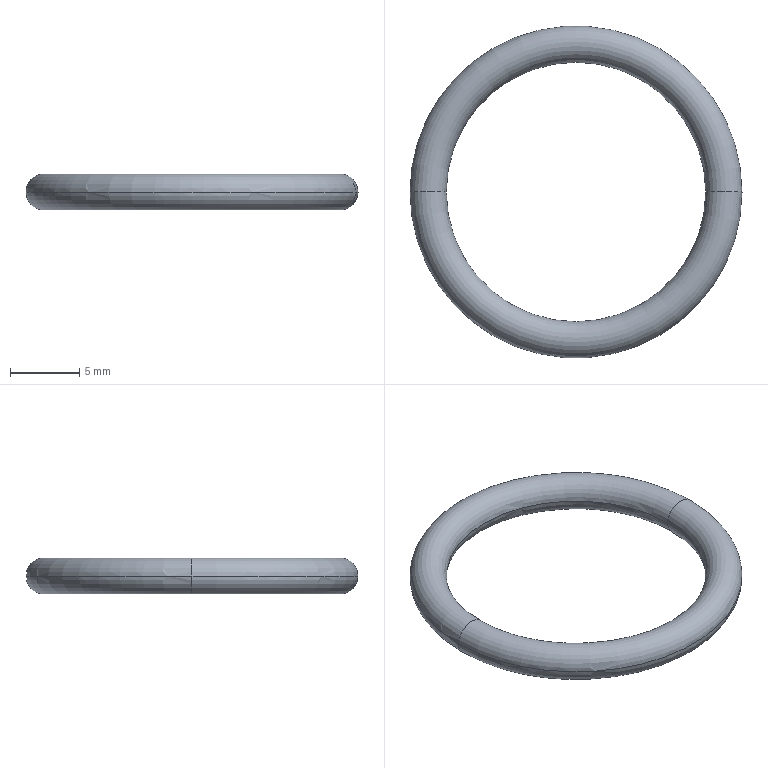Part | NX | features REVOLVE1 2 | 1 solid | 4 faces | box 23.952 x 23.952 x 2.616 mm | volume 360.325 mm3 | torus 4
STEP:
#1=CARTESIAN_POINT('',(-11.976,0.,0.));
#2=VERTEX_POINT('',#1);
#3=CARTESIAN_POINT('',(-9.36,0.,0.));
#4=VERTEX_POINT('',#3);
#5=CARTESIAN_POINT('',(-10.668,0.,0.));
#6=DIRECTION('',(0.,1.,0.));
#7=DIRECTION('',(-1.,0.,0.));
#8=AXIS2_PLACEMENT_3D('',#5,#6,#7);
#9=CIRCLE('',#8,1.308);
#10=EDGE_CURVE('',#2,#4,#9,.T.);
#11=ORIENTED_EDGE('',*,*,#10,.F.);
#12=CARTESIAN_POINT('',(11.976,0.,0.));
#13=VERTEX_POINT('',#12);
#14=CARTESIAN_POINT('',(0.,0.,0.));
#15=DIRECTION('',(0.,0.,1.));
#16=DIRECTION('',(1.,0.,0.));
#17=AXIS2_PLACEMENT_3D('',#14,#15,#16);
#18=CIRCLE('',#17,11.976);
#19=EDGE_CURVE('',#2,#13,#18,.T.);
#20=ORIENTED_EDGE('',*,*,#19,.T.);
#21=CARTESIAN_POINT('',(9.36,0.,0.));
#22=VERTEX_POINT('',#21);
#23=CARTESIAN_POINT('',(10.668,0.,0.));
#24=DIRECTION('',(0.,-1.,0.));
#25=DIRECTION('',(0.,0.,-1.));
#26=AXIS2_PLACEMENT_3D('',#23,#24,#25);
#27=CIRCLE('',#26,1.308);
#28=EDGE_CURVE('',#22,#13,#27,.F.);
#29=ORIENTED_EDGE('',*,*,#28,.F.);
#30=CARTESIAN_POINT('',(0.,0.,0.));
#31=DIRECTION('',(0.,0.,1.));
#32=DIRECTION('',(1.,0.,0.));
#33=AXIS2_PLACEMENT_3D('',#30,#31,#32);
#34=CIRCLE('',#33,9.36);
#35=EDGE_CURVE('',#22,#4,#34,.F.);
#36=ORIENTED_EDGE('',*,*,#35,.T.);
#37=EDGE_LOOP('',(#11,#20,#29,#36));
#38=FACE_BOUND('',#37,.T.);
#39=CARTESIAN_POINT('',(0.,0.,0.));
#40=DIRECTION('',(0.,0.,1.));
#41=DIRECTION('',(-1.,0.,0.));
#42=AXIS2_PLACEMENT_3D('',#39,#40,#41);
#43=TOROIDAL_SURFACE('',#42,10.668,1.308);
#44=ADVANCED_FACE('',(#38),#43,.T.);
#45=ORIENTED_EDGE('',*,*,#28,.T.);
#46=CARTESIAN_POINT('',(0.,0.,0.));
#47=DIRECTION('',(0.,0.,1.));
#48=DIRECTION('',(1.,0.,0.));
#49=AXIS2_PLACEMENT_3D('',#46,#47,#48);
#50=CIRCLE('',#49,11.976);
#51=EDGE_CURVE('',#13,#2,#50,.T.);
#52=ORIENTED_EDGE('',*,*,#51,.T.);
#53=ORIENTED_EDGE('',*,*,#10,.T.);
#54=CARTESIAN_POINT('',(0.,0.,0.));
#55=DIRECTION('',(0.,0.,1.));
#56=DIRECTION('',(1.,0.,0.));
#57=AXIS2_PLACEMENT_3D('',#54,#55,#56);
#58=CIRCLE('',#57,9.36);
#59=EDGE_CURVE('',#4,#22,#58,.F.);
#60=ORIENTED_EDGE('',*,*,#59,.T.);
#61=EDGE_LOOP('',(#45,#52,#53,#60));
#62=FACE_BOUND('',#61,.T.);
#63=CARTESIAN_POINT('',(0.,0.,0.));
#64=DIRECTION('',(0.,0.,1.));
#65=DIRECTION('',(-1.,0.,0.));
#66=AXIS2_PLACEMENT_3D('',#63,#64,#65);
#67=TOROIDAL_SURFACE('',#66,10.668,1.308);
#68=ADVANCED_FACE('',(#62),#67,.T.);
#69=ORIENTED_EDGE('',*,*,#51,.F.);
#70=CARTESIAN_POINT('',(10.668,0.,0.));
#71=DIRECTION('',(0.,-1.,0.));
#72=DIRECTION('',(0.,0.,-1.));
#73=AXIS2_PLACEMENT_3D('',#70,#71,#72);
#74=CIRCLE('',#73,1.308);
#75=EDGE_CURVE('',#13,#22,#74,.F.);
#76=ORIENTED_EDGE('',*,*,#75,.T.);
#77=ORIENTED_EDGE('',*,*,#59,.F.);
#78=CARTESIAN_POINT('',(-10.668,0.,0.));
#79=DIRECTION('',(0.,1.,0.));
#80=DIRECTION('',(-1.,0.,0.));
#81=AXIS2_PLACEMENT_3D('',#78,#79,#80);
#82=CIRCLE('',#81,1.308);
#83=EDGE_CURVE('',#4,#2,#82,.T.);
#84=ORIENTED_EDGE('',*,*,#83,.T.);
#85=EDGE_LOOP('',(#69,#76,#77,#84));
#86=FACE_BOUND('',#85,.T.);
#87=CARTESIAN_POINT('',(0.,0.,0.));
#88=DIRECTION('',(0.,0.,1.));
#89=DIRECTION('',(-1.,0.,0.));
#90=AXIS2_PLACEMENT_3D('',#87,#88,#89);
#91=TOROIDAL_SURFACE('',#90,10.668,1.308);
#92=ADVANCED_FACE('',(#86),#91,.T.);
#93=ORIENTED_EDGE('',*,*,#19,.F.);
#94=ORIENTED_EDGE('',*,*,#83,.F.);
#95=ORIENTED_EDGE('',*,*,#35,.F.);
#96=ORIENTED_EDGE('',*,*,#75,.F.);
#97=EDGE_LOOP('',(#93,#94,#95,#96));
#98=FACE_BOUND('',#97,.T.);
#99=CARTESIAN_POINT('',(0.,0.,0.));
#100=DIRECTION('',(0.,0.,1.));
#101=DIRECTION('',(-1.,0.,0.));
#102=AXIS2_PLACEMENT_3D('',#99,#100,#101);
#103=TOROIDAL_SURFACE('',#102,10.668,1.308);
#104=ADVANCED_FACE('',(#98),#103,.T.);
#105=CLOSED_SHELL('',(#44,#68,#92,#104));
#106=MANIFOLD_SOLID_BREP('',#105);
#107=(LENGTH_UNIT()NAMED_UNIT(*)SI_UNIT(.MILLI.,.METRE.));
#108=UNCERTAINTY_MEASURE_WITH_UNIT(LENGTH_MEASURE(0.00001),#107,'','');
#109=(NAMED_UNIT(*)PLANE_ANGLE_UNIT()SI_UNIT($,.RADIAN.));
#110=(NAMED_UNIT(*)SI_UNIT($,.STERADIAN.)SOLID_ANGLE_UNIT());
#111=(GEOMETRIC_REPRESENTATION_CONTEXT(3)GLOBAL_UNCERTAINTY_ASSIGNED_CONTEXT((#108))GLOBAL_UNIT_ASSIGNED_CONTEXT((#107,#109,#110))REPRESENTATION_CONTEXT('',''));
#112=ADVANCED_BREP_SHAPE_REPRESENTATION('',(#106),#111);